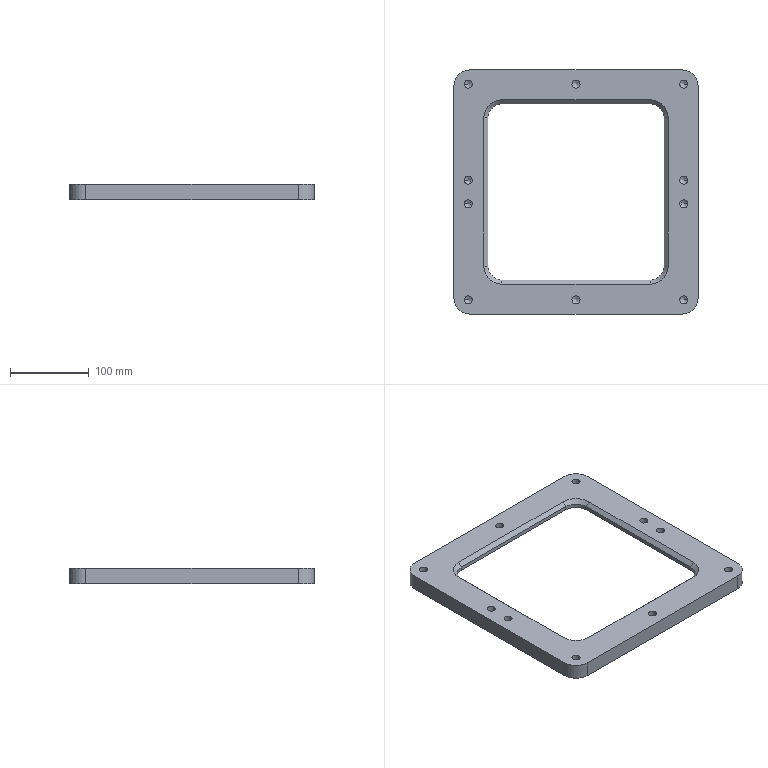Part | SolidWorks | features 3DProfileFeature 1, Chamfer 1, Extrusion 1, Fillet 1, HoleWzd 1, ICE 1 | 1 solid | 75 faces | box 310 x 310 x 20 mm | volume 773843 mm3 | cylinder 32 | cone 24 | plane 19 | commonest cylinder face diameters 10.2 x20 36 x4 40 x4 60 x4